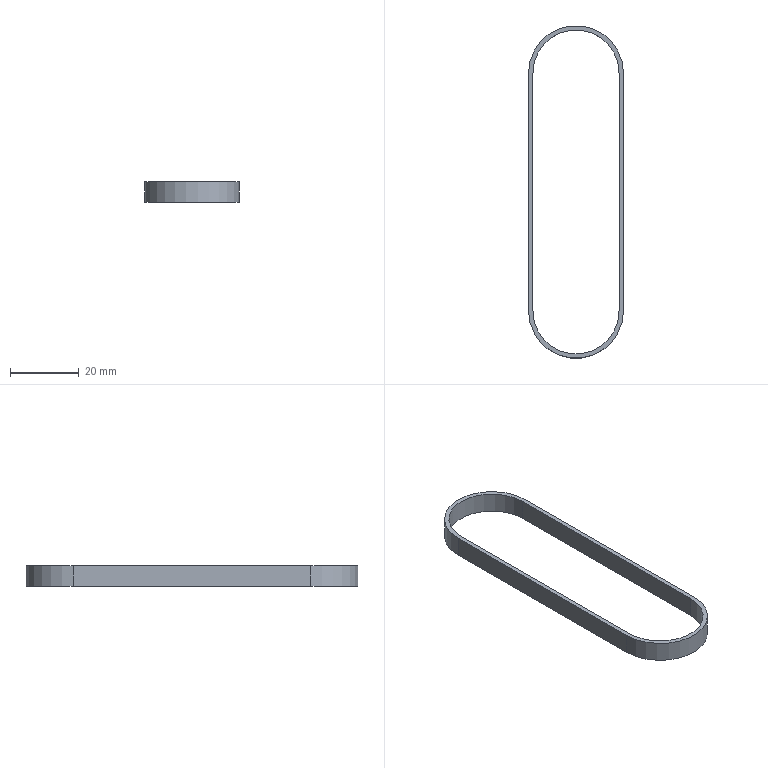Part | SolidWorks | features BaseBody 1 | 1 solid | 10 faces | box 27.5 x 96.5 x 6 mm | volume 1654 mm3 | plane 6 | cylinder 4 | commonest cylinder face diameters 25 x2 27.5 x2
STEP:
#1=CARTESIAN_POINT('',(12.5,0.,0.));
#2=VERTEX_POINT('',#1);
#3=CARTESIAN_POINT('',(12.5,0.,6.));
#4=VERTEX_POINT('',#3);
#5=CARTESIAN_POINT('',(12.5,0.,0.));
#6=DIRECTION('',(0.,0.,1.));
#7=VECTOR('',#6,1000.);
#8=LINE('',#5,#7);
#9=EDGE_CURVE('',#2,#4,#8,.T.);
#10=ORIENTED_EDGE('',*,*,#9,.F.);
#11=CARTESIAN_POINT('',(12.5,-69.,0.));
#12=VERTEX_POINT('',#11);
#13=CARTESIAN_POINT('',(12.5,0.,0.));
#14=DIRECTION('',(0.,1.,0.));
#15=VECTOR('',#14,1000.);
#16=LINE('',#13,#15);
#17=EDGE_CURVE('',#12,#2,#16,.T.);
#18=ORIENTED_EDGE('',*,*,#17,.F.);
#19=CARTESIAN_POINT('',(12.5,-69.,6.));
#20=VERTEX_POINT('',#19);
#21=CARTESIAN_POINT('',(12.5,-69.,0.));
#22=DIRECTION('',(0.,0.,-1.));
#23=VECTOR('',#22,1000.);
#24=LINE('',#21,#23);
#25=EDGE_CURVE('',#20,#12,#24,.T.);
#26=ORIENTED_EDGE('',*,*,#25,.F.);
#27=CARTESIAN_POINT('',(12.5,0.,6.));
#28=DIRECTION('',(0.,-1.,0.));
#29=VECTOR('',#28,1000.);
#30=LINE('',#27,#29);
#31=EDGE_CURVE('',#4,#20,#30,.T.);
#32=ORIENTED_EDGE('',*,*,#31,.F.);
#33=EDGE_LOOP('',(#10,#18,#26,#32));
#34=FACE_OUTER_BOUND('',#33,.T.);
#35=CARTESIAN_POINT('',(12.5,0.,0.));
#36=DIRECTION('',(1.,0.,0.));
#37=DIRECTION('',(0.,0.,-1.));
#38=AXIS2_PLACEMENT_3D('',#35,#36,#37);
#39=PLANE('',#38);
#40=ADVANCED_FACE('',(#34),#39,.F.);
#41=CARTESIAN_POINT('',(-12.5,-69.,6.));
#42=VERTEX_POINT('',#41);
#43=CARTESIAN_POINT('',(-12.5,0.,6.));
#44=VERTEX_POINT('',#43);
#45=CARTESIAN_POINT('',(-12.5,-34.5,6.));
#46=DIRECTION('',(0.,1.,0.));
#47=VECTOR('',#46,1000.);
#48=LINE('',#45,#47);
#49=EDGE_CURVE('',#42,#44,#48,.T.);
#50=ORIENTED_EDGE('',*,*,#49,.T.);
#51=CARTESIAN_POINT('',(0.,0.,6.));
#52=DIRECTION('',(0.,0.,-1.));
#53=DIRECTION('',(1.,0.,0.));
#54=AXIS2_PLACEMENT_3D('',#51,#52,#53);
#55=CIRCLE('',#54,12.5);
#56=EDGE_CURVE('',#44,#4,#55,.T.);
#57=ORIENTED_EDGE('',*,*,#56,.T.);
#58=ORIENTED_EDGE('',*,*,#31,.T.);
#59=CARTESIAN_POINT('',(0.,-69.,6.));
#60=DIRECTION('',(0.,0.,-1.));
#61=DIRECTION('',(1.,0.,0.));
#62=AXIS2_PLACEMENT_3D('',#59,#60,#61);
#63=CIRCLE('',#62,12.5);
#64=EDGE_CURVE('',#20,#42,#63,.T.);
#65=ORIENTED_EDGE('',*,*,#64,.T.);
#66=EDGE_LOOP('',(#50,#57,#58,#65));
#67=FACE_BOUND('',#66,.T.);
#68=CARTESIAN_POINT('',(-13.75,0.,6.));
#69=VERTEX_POINT('',#68);
#70=CARTESIAN_POINT('',(-13.75,-69.,6.));
#71=VERTEX_POINT('',#70);
#72=CARTESIAN_POINT('',(-13.75,-34.5,6.));
#73=DIRECTION('',(0.,-1.,0.));
#74=VECTOR('',#73,1000.);
#75=LINE('',#72,#74);
#76=EDGE_CURVE('',#69,#71,#75,.T.);
#77=ORIENTED_EDGE('',*,*,#76,.T.);
#78=CARTESIAN_POINT('',(13.75,-69.,6.));
#79=VERTEX_POINT('',#78);
#80=CARTESIAN_POINT('',(0.,-69.,6.));
#81=DIRECTION('',(0.,0.,1.));
#82=DIRECTION('',(1.,0.,0.));
#83=AXIS2_PLACEMENT_3D('',#80,#81,#82);
#84=CIRCLE('',#83,13.75);
#85=EDGE_CURVE('',#71,#79,#84,.T.);
#86=ORIENTED_EDGE('',*,*,#85,.T.);
#87=CARTESIAN_POINT('',(13.75,0.,6.));
#88=VERTEX_POINT('',#87);
#89=CARTESIAN_POINT('',(13.75,-34.5,6.));
#90=DIRECTION('',(0.,1.,0.));
#91=VECTOR('',#90,1000.);
#92=LINE('',#89,#91);
#93=EDGE_CURVE('',#79,#88,#92,.T.);
#94=ORIENTED_EDGE('',*,*,#93,.T.);
#95=CARTESIAN_POINT('',(0.,0.,6.));
#96=DIRECTION('',(0.,0.,1.));
#97=DIRECTION('',(1.,0.,0.));
#98=AXIS2_PLACEMENT_3D('',#95,#96,#97);
#99=CIRCLE('',#98,13.75);
#100=EDGE_CURVE('',#88,#69,#99,.T.);
#101=ORIENTED_EDGE('',*,*,#100,.T.);
#102=EDGE_LOOP('',(#77,#86,#94,#101));
#103=FACE_OUTER_BOUND('',#102,.T.);
#104=CARTESIAN_POINT('',(0.,-34.5,6.));
#105=DIRECTION('',(0.,0.,1.));
#106=DIRECTION('',(1.,0.,0.));
#107=AXIS2_PLACEMENT_3D('',#104,#105,#106);
#108=PLANE('',#107);
#109=ADVANCED_FACE('',(#67,#103),#108,.T.);
#110=CARTESIAN_POINT('',(-12.5,0.,0.));
#111=VERTEX_POINT('',#110);
#112=CARTESIAN_POINT('',(-12.5,0.,0.));
#113=DIRECTION('',(0.,0.,1.));
#114=VECTOR('',#113,1000.);
#115=LINE('',#112,#114);
#116=EDGE_CURVE('',#111,#44,#115,.T.);
#117=ORIENTED_EDGE('',*,*,#116,.F.);
#118=CARTESIAN_POINT('',(0.,0.,0.));
#119=DIRECTION('',(0.,0.,1.));
#120=DIRECTION('',(1.,0.,0.));
#121=AXIS2_PLACEMENT_3D('',#118,#119,#120);
#122=CIRCLE('',#121,12.5);
#123=EDGE_CURVE('',#2,#111,#122,.T.);
#124=ORIENTED_EDGE('',*,*,#123,.F.);
#125=ORIENTED_EDGE('',*,*,#9,.T.);
#126=ORIENTED_EDGE('',*,*,#56,.F.);
#127=EDGE_LOOP('',(#117,#124,#125,#126));
#128=FACE_OUTER_BOUND('',#127,.T.);
#129=CARTESIAN_POINT('',(0.,0.,0.));
#130=DIRECTION('',(0.,0.,1.));
#131=DIRECTION('',(1.,0.,0.));
#132=AXIS2_PLACEMENT_3D('',#129,#130,#131);
#133=CYLINDRICAL_SURFACE('',#132,12.5);
#134=ADVANCED_FACE('',(#128),#133,.F.);
#135=ORIENTED_EDGE('',*,*,#123,.T.);
#136=CARTESIAN_POINT('',(-12.5,-69.,0.));
#137=VERTEX_POINT('',#136);
#138=CARTESIAN_POINT('',(-12.5,-34.5,0.));
#139=DIRECTION('',(0.,1.,0.));
#140=VECTOR('',#139,1000.);
#141=LINE('',#138,#140);
#142=EDGE_CURVE('',#137,#111,#141,.T.);
#143=ORIENTED_EDGE('',*,*,#142,.F.);
#144=CARTESIAN_POINT('',(0.,-69.,0.));
#145=DIRECTION('',(0.,0.,-1.));
#146=DIRECTION('',(1.,0.,0.));
#147=AXIS2_PLACEMENT_3D('',#144,#145,#146);
#148=CIRCLE('',#147,12.5);
#149=EDGE_CURVE('',#12,#137,#148,.T.);
#150=ORIENTED_EDGE('',*,*,#149,.F.);
#151=ORIENTED_EDGE('',*,*,#17,.T.);
#152=EDGE_LOOP('',(#135,#143,#150,#151));
#153=FACE_BOUND('',#152,.T.);
#154=CARTESIAN_POINT('',(13.75,-69.,0.));
#155=VERTEX_POINT('',#154);
#156=CARTESIAN_POINT('',(13.75,0.,0.));
#157=VERTEX_POINT('',#156);
#158=CARTESIAN_POINT('',(13.75,-34.5,0.));
#159=DIRECTION('',(0.,1.,0.));
#160=VECTOR('',#159,1000.);
#161=LINE('',#158,#160);
#162=EDGE_CURVE('',#155,#157,#161,.T.);
#163=ORIENTED_EDGE('',*,*,#162,.F.);
#164=CARTESIAN_POINT('',(-13.75,-69.,0.));
#165=VERTEX_POINT('',#164);
#166=CARTESIAN_POINT('',(0.,-69.,0.));
#167=DIRECTION('',(0.,0.,1.));
#168=DIRECTION('',(1.,0.,0.));
#169=AXIS2_PLACEMENT_3D('',#166,#167,#168);
#170=CIRCLE('',#169,13.75);
#171=EDGE_CURVE('',#165,#155,#170,.T.);
#172=ORIENTED_EDGE('',*,*,#171,.F.);
#173=CARTESIAN_POINT('',(-13.75,0.,0.));
#174=VERTEX_POINT('',#173);
#175=CARTESIAN_POINT('',(-13.75,-34.5,0.));
#176=DIRECTION('',(0.,-1.,0.));
#177=VECTOR('',#176,1000.);
#178=LINE('',#175,#177);
#179=EDGE_CURVE('',#174,#165,#178,.T.);
#180=ORIENTED_EDGE('',*,*,#179,.F.);
#181=CARTESIAN_POINT('',(0.,0.,0.));
#182=DIRECTION('',(0.,0.,1.));
#183=DIRECTION('',(1.,0.,0.));
#184=AXIS2_PLACEMENT_3D('',#181,#182,#183);
#185=CIRCLE('',#184,13.75);
#186=EDGE_CURVE('',#157,#174,#185,.T.);
#187=ORIENTED_EDGE('',*,*,#186,.F.);
#188=EDGE_LOOP('',(#163,#172,#180,#187));
#189=FACE_OUTER_BOUND('',#188,.T.);
#190=CARTESIAN_POINT('',(0.,-34.5,0.));
#191=DIRECTION('',(0.,0.,1.));
#192=DIRECTION('',(1.,0.,0.));
#193=AXIS2_PLACEMENT_3D('',#190,#191,#192);
#194=PLANE('',#193);
#195=ADVANCED_FACE('',(#153,#189),#194,.F.);
#196=ORIENTED_EDGE('',*,*,#25,.T.);
#197=ORIENTED_EDGE('',*,*,#149,.T.);
#198=CARTESIAN_POINT('',(-12.5,-69.,0.));
#199=DIRECTION('',(0.,0.,-1.));
#200=VECTOR('',#199,1000.);
#201=LINE('',#198,#200);
#202=EDGE_CURVE('',#42,#137,#201,.T.);
#203=ORIENTED_EDGE('',*,*,#202,.F.);
#204=ORIENTED_EDGE('',*,*,#64,.F.);
#205=EDGE_LOOP('',(#196,#197,#203,#204));
#206=FACE_OUTER_BOUND('',#205,.T.);
#207=CARTESIAN_POINT('',(0.,-69.,0.));
#208=DIRECTION('',(0.,0.,1.));
#209=DIRECTION('',(1.,0.,0.));
#210=AXIS2_PLACEMENT_3D('',#207,#208,#209);
#211=CYLINDRICAL_SURFACE('',#210,12.5);
#212=ADVANCED_FACE('',(#206),#211,.F.);
#213=ORIENTED_EDGE('',*,*,#202,.T.);
#214=ORIENTED_EDGE('',*,*,#142,.T.);
#215=ORIENTED_EDGE('',*,*,#116,.T.);
#216=ORIENTED_EDGE('',*,*,#49,.F.);
#217=EDGE_LOOP('',(#213,#214,#215,#216));
#218=FACE_OUTER_BOUND('',#217,.T.);
#219=CARTESIAN_POINT('',(-12.5,-69.,0.));
#220=DIRECTION('',(-1.,0.,0.));
#221=DIRECTION('',(0.,0.,1.));
#222=AXIS2_PLACEMENT_3D('',#219,#220,#221);
#223=PLANE('',#222);
#224=ADVANCED_FACE('',(#218),#223,.F.);
#225=ORIENTED_EDGE('',*,*,#171,.T.);
#226=CARTESIAN_POINT('',(13.75,-69.,0.));
#227=DIRECTION('',(0.,0.,1.));
#228=VECTOR('',#227,1000.);
#229=LINE('',#226,#228);
#230=EDGE_CURVE('',#155,#79,#229,.T.);
#231=ORIENTED_EDGE('',*,*,#230,.T.);
#232=ORIENTED_EDGE('',*,*,#85,.F.);
#233=CARTESIAN_POINT('',(-13.75,-69.,0.));
#234=DIRECTION('',(0.,0.,-1.));
#235=VECTOR('',#234,1000.);
#236=LINE('',#233,#235);
#237=EDGE_CURVE('',#71,#165,#236,.T.);
#238=ORIENTED_EDGE('',*,*,#237,.T.);
#239=EDGE_LOOP('',(#225,#231,#232,#238));
#240=FACE_OUTER_BOUND('',#239,.T.);
#241=CARTESIAN_POINT('',(0.,-69.,0.));
#242=DIRECTION('',(0.,0.,1.));
#243=DIRECTION('',(1.,0.,0.));
#244=AXIS2_PLACEMENT_3D('',#241,#242,#243);
#245=CYLINDRICAL_SURFACE('',#244,13.75);
#246=ADVANCED_FACE('',(#240),#245,.T.);
#247=ORIENTED_EDGE('',*,*,#179,.T.);
#248=ORIENTED_EDGE('',*,*,#237,.F.);
#249=ORIENTED_EDGE('',*,*,#76,.F.);
#250=CARTESIAN_POINT('',(-13.75,0.,0.));
#251=DIRECTION('',(0.,0.,-1.));
#252=VECTOR('',#251,1000.);
#253=LINE('',#250,#252);
#254=EDGE_CURVE('',#69,#174,#253,.T.);
#255=ORIENTED_EDGE('',*,*,#254,.T.);
#256=EDGE_LOOP('',(#247,#248,#249,#255));
#257=FACE_OUTER_BOUND('',#256,.T.);
#258=CARTESIAN_POINT('',(-13.75,-69.,0.));
#259=DIRECTION('',(-1.,0.,0.));
#260=DIRECTION('',(0.,0.,1.));
#261=AXIS2_PLACEMENT_3D('',#258,#259,#260);
#262=PLANE('',#261);
#263=ADVANCED_FACE('',(#257),#262,.T.);
#264=ORIENTED_EDGE('',*,*,#186,.T.);
#265=ORIENTED_EDGE('',*,*,#254,.F.);
#266=ORIENTED_EDGE('',*,*,#100,.F.);
#267=CARTESIAN_POINT('',(13.75,0.,0.));
#268=DIRECTION('',(0.,0.,-1.));
#269=VECTOR('',#268,1000.);
#270=LINE('',#267,#269);
#271=EDGE_CURVE('',#88,#157,#270,.T.);
#272=ORIENTED_EDGE('',*,*,#271,.T.);
#273=EDGE_LOOP('',(#264,#265,#266,#272));
#274=FACE_OUTER_BOUND('',#273,.T.);
#275=CARTESIAN_POINT('',(0.,0.,0.));
#276=DIRECTION('',(0.,0.,1.));
#277=DIRECTION('',(1.,0.,0.));
#278=AXIS2_PLACEMENT_3D('',#275,#276,#277);
#279=CYLINDRICAL_SURFACE('',#278,13.75);
#280=ADVANCED_FACE('',(#274),#279,.T.);
#281=ORIENTED_EDGE('',*,*,#162,.T.);
#282=ORIENTED_EDGE('',*,*,#271,.F.);
#283=ORIENTED_EDGE('',*,*,#93,.F.);
#284=ORIENTED_EDGE('',*,*,#230,.F.);
#285=EDGE_LOOP('',(#281,#282,#283,#284));
#286=FACE_OUTER_BOUND('',#285,.T.);
#287=CARTESIAN_POINT('',(13.75,0.,0.));
#288=DIRECTION('',(1.,0.,0.));
#289=DIRECTION('',(0.,0.,-1.));
#290=AXIS2_PLACEMENT_3D('',#287,#288,#289);
#291=PLANE('',#290);
#292=ADVANCED_FACE('',(#286),#291,.T.);
#293=CLOSED_SHELL('',(#40,#109,#134,#195,#212,#224,#246,#263,#280,#292));
#294=MANIFOLD_SOLID_BREP('',#293);
#295=CARTESIAN_POINT('',(0.,0.,0.));
#296=DIRECTION('',(0.,0.,1.));
#297=DIRECTION('',(1.,0.,0.));
#298=AXIS2_PLACEMENT_3D('',#295,#296,#297);
#299=(LENGTH_UNIT()NAMED_UNIT(*)SI_UNIT(.MILLI.,.METRE.));
#300=UNCERTAINTY_MEASURE_WITH_UNIT(LENGTH_MEASURE(0.00001),#299,'','');
#301=(NAMED_UNIT(*)PLANE_ANGLE_UNIT()SI_UNIT($,.RADIAN.));
#302=(NAMED_UNIT(*)SI_UNIT($,.STERADIAN.)SOLID_ANGLE_UNIT());
#303=(GEOMETRIC_REPRESENTATION_CONTEXT(3)GLOBAL_UNCERTAINTY_ASSIGNED_CONTEXT((#300))GLOBAL_UNIT_ASSIGNED_CONTEXT((#299,#301,#302))REPRESENTATION_CONTEXT('',''));
#304=ADVANCED_BREP_SHAPE_REPRESENTATION('',(#294,#298),#303);